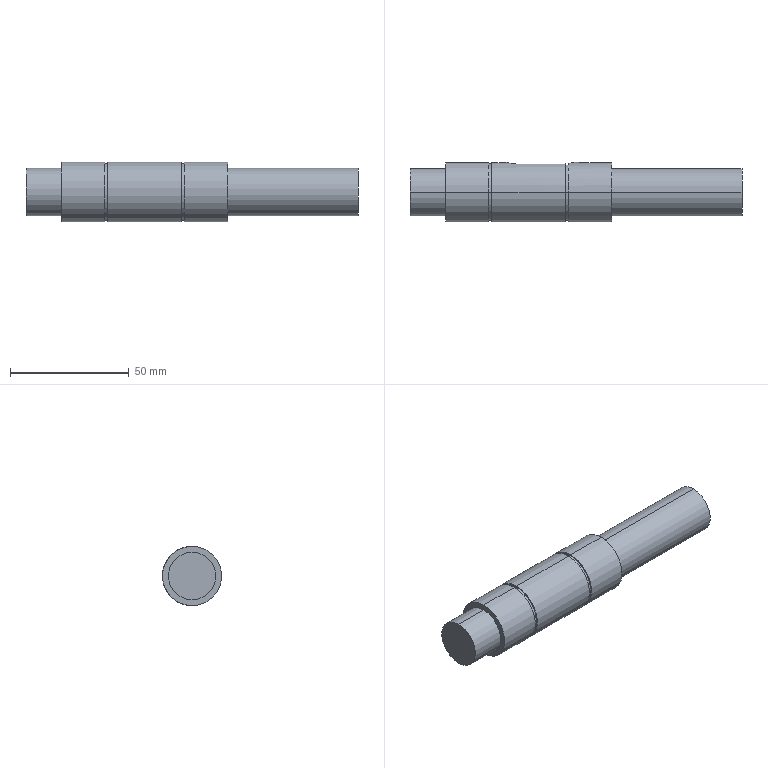Part | SolidWorks | features ICE 3, Extrusion 1, RevCut 1 | 1 solid | 28 faces | box 140 x 25 x 25 mm | volume 55450 mm3 | cylinder 17 | plane 11 | commonest cylinder face diameters 25 x6 23.9 x5 20 x4 8 x2
STEP:
#1=CARTESIAN_POINT('',(-50.,0.,10.));
#2=VERTEX_POINT('',#1);
#3=CARTESIAN_POINT('',(-50.,0.,-10.));
#4=VERTEX_POINT('',#3);
#5=CARTESIAN_POINT('',(-50.,0.,0.));
#6=DIRECTION('',(-1.,0.,0.));
#7=DIRECTION('',(0.,0.,1.));
#8=AXIS2_PLACEMENT_3D('',#5,#6,#7);
#9=CIRCLE('',#8,10.);
#10=EDGE_CURVE('',#2,#4,#9,.T.);
#11=ORIENTED_EDGE('',*,*,#10,.F.);
#12=CARTESIAN_POINT('',(-35.,0.,10.));
#13=VERTEX_POINT('',#12);
#14=CARTESIAN_POINT('',(-50.,0.,10.));
#15=DIRECTION('',(1.,0.,0.));
#16=VECTOR('',#15,1000.);
#17=LINE('',#14,#16);
#18=EDGE_CURVE('',#2,#13,#17,.T.);
#19=ORIENTED_EDGE('',*,*,#18,.T.);
#20=CARTESIAN_POINT('',(-35.,0.,-10.));
#21=VERTEX_POINT('',#20);
#22=CARTESIAN_POINT('',(-35.,0.,0.));
#23=DIRECTION('',(-1.,0.,0.));
#24=DIRECTION('',(0.,0.,1.));
#25=AXIS2_PLACEMENT_3D('',#22,#23,#24);
#26=CIRCLE('',#25,10.);
#27=EDGE_CURVE('',#13,#21,#26,.T.);
#28=ORIENTED_EDGE('',*,*,#27,.T.);
#29=CARTESIAN_POINT('',(-50.,0.,-10.));
#30=DIRECTION('',(1.,0.,0.));
#31=VECTOR('',#30,1000.);
#32=LINE('',#29,#31);
#33=EDGE_CURVE('',#4,#21,#32,.T.);
#34=ORIENTED_EDGE('',*,*,#33,.F.);
#35=EDGE_LOOP('',(#11,#19,#28,#34));
#36=FACE_OUTER_BOUND('',#35,.T.);
#37=CARTESIAN_POINT('',(-50.,0.,0.));
#38=DIRECTION('',(1.,0.,0.));
#39=DIRECTION('',(0.,0.,-1.));
#40=AXIS2_PLACEMENT_3D('',#37,#38,#39);
#41=CYLINDRICAL_SURFACE('',#40,10.);
#42=ADVANCED_FACE('',(#36),#41,.T.);
#43=CARTESIAN_POINT('',(-16.8,0.,12.5));
#44=VERTEX_POINT('',#43);
#45=CARTESIAN_POINT('',(-16.8,0.,-12.5));
#46=VERTEX_POINT('',#45);
#47=CARTESIAN_POINT('',(-16.8,0.,0.));
#48=DIRECTION('',(-1.,0.,0.));
#49=DIRECTION('',(0.,0.,1.));
#50=AXIS2_PLACEMENT_3D('',#47,#48,#49);
#51=CIRCLE('',#50,12.5);
#52=EDGE_CURVE('',#44,#46,#51,.T.);
#53=ORIENTED_EDGE('',*,*,#52,.T.);
#54=CARTESIAN_POINT('',(-35.,0.,-12.5));
#55=VERTEX_POINT('',#54);
#56=CARTESIAN_POINT('',(35.,0.,-12.5));
#57=DIRECTION('',(-1.,0.,0.));
#58=VECTOR('',#57,1000.);
#59=LINE('',#56,#58);
#60=EDGE_CURVE('',#46,#55,#59,.T.);
#61=ORIENTED_EDGE('',*,*,#60,.T.);
#62=CARTESIAN_POINT('',(-35.,0.,12.5));
#63=VERTEX_POINT('',#62);
#64=CARTESIAN_POINT('',(-35.,0.,0.));
#65=DIRECTION('',(1.,0.,0.));
#66=DIRECTION('',(0.,0.,-1.));
#67=AXIS2_PLACEMENT_3D('',#64,#65,#66);
#68=CIRCLE('',#67,12.5);
#69=EDGE_CURVE('',#55,#63,#68,.T.);
#70=ORIENTED_EDGE('',*,*,#69,.T.);
#71=CARTESIAN_POINT('',(35.,0.,12.5));
#72=DIRECTION('',(-1.,0.,0.));
#73=VECTOR('',#72,1000.);
#74=LINE('',#71,#73);
#75=EDGE_CURVE('',#44,#63,#74,.T.);
#76=ORIENTED_EDGE('',*,*,#75,.F.);
#77=EDGE_LOOP('',(#53,#61,#70,#76));
#78=FACE_OUTER_BOUND('',#77,.T.);
#79=CARTESIAN_POINT('',(35.,0.,0.));
#80=DIRECTION('',(-1.,0.,0.));
#81=DIRECTION('',(0.,0.,1.));
#82=AXIS2_PLACEMENT_3D('',#79,#80,#81);
#83=CYLINDRICAL_SURFACE('',#82,12.5);
#84=ADVANCED_FACE('',(#78),#83,.T.);
#85=CARTESIAN_POINT('',(-15.5,0.,11.95));
#86=VERTEX_POINT('',#85);
#87=CARTESIAN_POINT('',(-15.5,0.,-11.95));
#88=VERTEX_POINT('',#87);
#89=CARTESIAN_POINT('',(-15.5,0.,0.));
#90=DIRECTION('',(-1.,0.,0.));
#91=DIRECTION('',(0.,0.,1.));
#92=AXIS2_PLACEMENT_3D('',#89,#90,#91);
#93=CIRCLE('',#92,11.95);
#94=EDGE_CURVE('',#86,#88,#93,.T.);
#95=ORIENTED_EDGE('',*,*,#94,.T.);
#96=CARTESIAN_POINT('',(-16.8,0.,-11.95));
#97=VERTEX_POINT('',#96);
#98=CARTESIAN_POINT('',(0.,0.,-11.95));
#99=DIRECTION('',(-1.,0.,0.));
#100=VECTOR('',#99,1000.);
#101=LINE('',#98,#100);
#102=EDGE_CURVE('',#88,#97,#101,.T.);
#103=ORIENTED_EDGE('',*,*,#102,.T.);
#104=CARTESIAN_POINT('',(-16.8,0.,11.95));
#105=VERTEX_POINT('',#104);
#106=CARTESIAN_POINT('',(-16.8,0.,0.));
#107=DIRECTION('',(-1.,0.,0.));
#108=DIRECTION('',(0.,0.,1.));
#109=AXIS2_PLACEMENT_3D('',#106,#107,#108);
#110=CIRCLE('',#109,11.95);
#111=EDGE_CURVE('',#105,#97,#110,.T.);
#112=ORIENTED_EDGE('',*,*,#111,.F.);
#113=CARTESIAN_POINT('',(0.,0.,11.95));
#114=DIRECTION('',(-1.,0.,0.));
#115=VECTOR('',#114,1000.);
#116=LINE('',#113,#115);
#117=EDGE_CURVE('',#86,#105,#116,.T.);
#118=ORIENTED_EDGE('',*,*,#117,.F.);
#119=EDGE_LOOP('',(#95,#103,#112,#118));
#120=FACE_OUTER_BOUND('',#119,.T.);
#121=CARTESIAN_POINT('',(0.,0.,0.));
#122=DIRECTION('',(-1.,0.,0.));
#123=DIRECTION('',(0.,0.,1.));
#124=AXIS2_PLACEMENT_3D('',#121,#122,#123);
#125=CYLINDRICAL_SURFACE('',#124,11.95);
#126=ADVANCED_FACE('',(#120),#125,.T.);
#127=CARTESIAN_POINT('',(90.,0.,-10.));
#128=VERTEX_POINT('',#127);
#129=CARTESIAN_POINT('',(90.,0.,10.));
#130=VERTEX_POINT('',#129);
#131=CARTESIAN_POINT('',(90.,0.,0.));
#132=DIRECTION('',(1.,0.,0.));
#133=DIRECTION('',(0.,0.,-1.));
#134=AXIS2_PLACEMENT_3D('',#131,#132,#133);
#135=CIRCLE('',#134,10.);
#136=EDGE_CURVE('',#128,#130,#135,.T.);
#137=ORIENTED_EDGE('',*,*,#136,.F.);
#138=CARTESIAN_POINT('',(35.,0.,-10.));
#139=VERTEX_POINT('',#138);
#140=CARTESIAN_POINT('',(90.,0.,-10.));
#141=DIRECTION('',(-1.,0.,0.));
#142=VECTOR('',#141,1000.);
#143=LINE('',#140,#142);
#144=EDGE_CURVE('',#128,#139,#143,.T.);
#145=ORIENTED_EDGE('',*,*,#144,.T.);
#146=CARTESIAN_POINT('',(35.,0.,10.));
#147=VERTEX_POINT('',#146);
#148=CARTESIAN_POINT('',(35.,0.,0.));
#149=DIRECTION('',(1.,0.,0.));
#150=DIRECTION('',(0.,0.,-1.));
#151=AXIS2_PLACEMENT_3D('',#148,#149,#150);
#152=CIRCLE('',#151,10.);
#153=EDGE_CURVE('',#139,#147,#152,.T.);
#154=ORIENTED_EDGE('',*,*,#153,.T.);
#155=CARTESIAN_POINT('',(90.,0.,10.));
#156=DIRECTION('',(-1.,0.,0.));
#157=VECTOR('',#156,1000.);
#158=LINE('',#155,#157);
#159=EDGE_CURVE('',#130,#147,#158,.T.);
#160=ORIENTED_EDGE('',*,*,#159,.F.);
#161=EDGE_LOOP('',(#137,#145,#154,#160));
#162=FACE_OUTER_BOUND('',#161,.T.);
#163=CARTESIAN_POINT('',(90.,0.,0.));
#164=DIRECTION('',(-1.,0.,0.));
#165=DIRECTION('',(0.,0.,1.));
#166=AXIS2_PLACEMENT_3D('',#163,#164,#165);
#167=CYLINDRICAL_SURFACE('',#166,10.);
#168=ADVANCED_FACE('',(#162),#167,.T.);
#169=CARTESIAN_POINT('',(15.5,11.853,-3.969));
#170=VERTEX_POINT('',#169);
#171=CARTESIAN_POINT('',(15.5,0.,-12.5));
#172=VERTEX_POINT('',#171);
#173=CARTESIAN_POINT('',(15.5,0.,0.));
#174=DIRECTION('',(-1.,0.,0.));
#175=DIRECTION('',(0.,0.,1.));
#176=AXIS2_PLACEMENT_3D('',#173,#174,#175);
#177=CIRCLE('',#176,12.5);
#178=EDGE_CURVE('',#170,#172,#177,.T.);
#179=ORIENTED_EDGE('',*,*,#178,.T.);
#180=CARTESIAN_POINT('',(-15.5,0.,-12.5));
#181=VERTEX_POINT('',#180);
#182=CARTESIAN_POINT('',(35.,0.,-12.5));
#183=DIRECTION('',(-1.,0.,0.));
#184=VECTOR('',#183,1000.);
#185=LINE('',#182,#184);
#186=EDGE_CURVE('',#172,#181,#185,.T.);
#187=ORIENTED_EDGE('',*,*,#186,.T.);
#188=CARTESIAN_POINT('',(-15.5,0.,12.5));
#189=VERTEX_POINT('',#188);
#190=CARTESIAN_POINT('',(-15.5,0.,0.));
#191=DIRECTION('',(-1.,0.,0.));
#192=DIRECTION('',(0.,0.,1.));
#193=AXIS2_PLACEMENT_3D('',#190,#191,#192);
#194=CIRCLE('',#193,12.5);
#195=EDGE_CURVE('',#189,#181,#194,.T.);
#196=ORIENTED_EDGE('',*,*,#195,.F.);
#197=CARTESIAN_POINT('',(15.5,0.,12.5));
#198=VERTEX_POINT('',#197);
#199=CARTESIAN_POINT('',(35.,0.,12.5));
#200=DIRECTION('',(-1.,0.,0.));
#201=VECTOR('',#200,1000.);
#202=LINE('',#199,#201);
#203=EDGE_CURVE('',#198,#189,#202,.T.);
#204=ORIENTED_EDGE('',*,*,#203,.F.);
#205=CARTESIAN_POINT('',(15.5,11.853,3.969));
#206=VERTEX_POINT('',#205);
#207=CARTESIAN_POINT('',(15.5,0.,0.));
#208=DIRECTION('',(-1.,0.,0.));
#209=DIRECTION('',(0.,0.,1.));
#210=AXIS2_PLACEMENT_3D('',#207,#208,#209);
#211=CIRCLE('',#210,12.5);
#212=EDGE_CURVE('',#198,#206,#211,.T.);
#213=ORIENTED_EDGE('',*,*,#212,.T.);
#214=CARTESIAN_POINT('',(15.,11.843,4.));
#215=VERTEX_POINT('',#214);
#216=CARTESIAN_POINT('',(15.,11.843,4.));
#217=CARTESIAN_POINT('',(15.167,11.843,4.));
#218=CARTESIAN_POINT('',(15.334,11.846,3.99));
#219=CARTESIAN_POINT('',(15.5,11.853,3.969));
#220=B_SPLINE_CURVE_WITH_KNOTS('',3,(#216,#217,#218,#219),.UNSPECIFIED.,.F.,.F.,(4,4),(0.,0.0005011),.UNSPECIFIED.);
#221=EDGE_CURVE('',#215,#206,#220,.T.);
#222=ORIENTED_EDGE('',*,*,#221,.F.);
#223=CARTESIAN_POINT('',(-5.,11.843,4.));
#224=VERTEX_POINT('',#223);
#225=CARTESIAN_POINT('',(35.,11.843,4.));
#226=DIRECTION('',(1.,0.,0.));
#227=VECTOR('',#226,1000.);
#228=LINE('',#225,#227);
#229=EDGE_CURVE('',#224,#215,#228,.T.);
#230=ORIENTED_EDGE('',*,*,#229,.F.);
#231=CARTESIAN_POINT('',(-5.,11.843,-4.));
#232=VERTEX_POINT('',#231);
#233=CARTESIAN_POINT('',(-5.,11.843,-4.));
#234=CARTESIAN_POINT('',(-5.266,11.843,-4.));
#235=CARTESIAN_POINT('',(-5.527,11.852,-3.974));
#236=CARTESIAN_POINT('',(-6.041,11.886,-3.871));
#237=CARTESIAN_POINT('',(-6.296,11.911,-3.793));
#238=CARTESIAN_POINT('',(-6.779,11.973,-3.592));
#239=CARTESIAN_POINT('',(-7.008,12.01,-3.469));
#240=CARTESIAN_POINT('',(-7.441,12.09,-3.179));
#241=CARTESIAN_POINT('',(-7.645,12.133,-3.012));
#242=CARTESIAN_POINT('',(-8.011,12.218,-2.646));
#243=CARTESIAN_POINT('',(-8.176,12.26,-2.445));
#244=CARTESIAN_POINT('',(-8.469,12.34,-2.009));
#245=CARTESIAN_POINT('',(-8.592,12.375,-1.779));
#246=CARTESIAN_POINT('',(-8.792,12.435,-1.299));
#247=CARTESIAN_POINT('',(-8.87,12.459,-1.045));
#248=CARTESIAN_POINT('',(-8.974,12.492,-0.5276));
#249=CARTESIAN_POINT('',(-9.,12.5,-0.2669));
#250=CARTESIAN_POINT('',(-9.,12.5,0.2587));
#251=CARTESIAN_POINT('',(-8.974,12.492,0.5256));
#252=CARTESIAN_POINT('',(-8.871,12.459,1.04));
#253=CARTESIAN_POINT('',(-8.795,12.436,1.29));
#254=CARTESIAN_POINT('',(-8.593,12.375,1.777));
#255=CARTESIAN_POINT('',(-8.469,12.34,2.008));
#256=CARTESIAN_POINT('',(-8.18,12.262,2.44));
#257=CARTESIAN_POINT('',(-8.013,12.219,2.643));
#258=CARTESIAN_POINT('',(-7.645,12.133,3.012));
#259=CARTESIAN_POINT('',(-7.445,12.091,3.176));
#260=CARTESIAN_POINT('',(-7.013,12.011,3.466));
#261=CARTESIAN_POINT('',(-6.78,11.973,3.592));
#262=CARTESIAN_POINT('',(-6.298,11.911,3.792));
#263=CARTESIAN_POINT('',(-6.049,11.886,3.869));
#264=CARTESIAN_POINT('',(-5.532,11.852,3.973));
#265=CARTESIAN_POINT('',(-5.266,11.843,4.));
#266=CARTESIAN_POINT('',(-5.,11.843,4.));
#267=B_SPLINE_CURVE_WITH_KNOTS('',3,(#233,#234,#235,#236,#237,#238,#239,#240,#241,#242,#243,#244,#245,#246,#247,#248,#249,#250,#251,#252,#253,#254,#255,#256,#257,#258,#259,#260,#261,#262,#263,#264,#265,#266),.UNSPECIFIED.,.F.,.F.,(4,2,2,2,2,2,2,2,2,2,2,2,2,2,2,2,4),(0.,0.0007865,0.001573,0.00236,0.003146,0.003933,0.004719,0.005506,0.006292,0.007079,0.007865,0.008652,0.009438,0.01022,0.01101,0.0118,0.01258),.UNSPECIFIED.);
#268=EDGE_CURVE('',#232,#224,#267,.T.);
#269=ORIENTED_EDGE('',*,*,#268,.F.);
#270=CARTESIAN_POINT('',(15.,11.843,-4.));
#271=VERTEX_POINT('',#270);
#272=CARTESIAN_POINT('',(35.,11.843,-4.));
#273=DIRECTION('',(-1.,0.,0.));
#274=VECTOR('',#273,1000.);
#275=LINE('',#272,#274);
#276=EDGE_CURVE('',#271,#232,#275,.T.);
#277=ORIENTED_EDGE('',*,*,#276,.F.);
#278=CARTESIAN_POINT('',(15.5,11.853,-3.969));
#279=CARTESIAN_POINT('',(15.334,11.846,-3.99));
#280=CARTESIAN_POINT('',(15.167,11.843,-4.));
#281=CARTESIAN_POINT('',(15.,11.843,-4.));
#282=B_SPLINE_CURVE_WITH_KNOTS('',3,(#278,#279,#280,#281),.UNSPECIFIED.,.F.,.F.,(4,4),(0.,0.0005011),.UNSPECIFIED.);
#283=EDGE_CURVE('',#170,#271,#282,.T.);
#284=ORIENTED_EDGE('',*,*,#283,.F.);
#285=EDGE_LOOP('',(#179,#187,#196,#204,#213,#222,#230,#269,#277,#284));
#286=FACE_OUTER_BOUND('',#285,.T.);
#287=CARTESIAN_POINT('',(35.,0.,0.));
#288=DIRECTION('',(-1.,0.,0.));
#289=DIRECTION('',(0.,0.,1.));
#290=AXIS2_PLACEMENT_3D('',#287,#288,#289);
#291=CYLINDRICAL_SURFACE('',#290,12.5);
#292=ADVANCED_FACE('',(#286),#291,.T.);
#293=CARTESIAN_POINT('',(16.8,11.404,-3.572));
#294=VERTEX_POINT('',#293);
#295=CARTESIAN_POINT('',(16.8,0.,-11.95));
#296=VERTEX_POINT('',#295);
#297=CARTESIAN_POINT('',(16.8,0.,0.));
#298=DIRECTION('',(-1.,0.,0.));
#299=DIRECTION('',(0.,0.,1.));
#300=AXIS2_PLACEMENT_3D('',#297,#298,#299);
#301=CIRCLE('',#300,11.95);
#302=EDGE_CURVE('',#294,#296,#301,.T.);
#303=ORIENTED_EDGE('',*,*,#302,.T.);
#304=CARTESIAN_POINT('',(15.5,0.,-11.95));
#305=VERTEX_POINT('',#304);
#306=CARTESIAN_POINT('',(0.,0.,-11.95));
#307=DIRECTION('',(-1.,0.,0.));
#308=VECTOR('',#307,1000.);
#309=LINE('',#306,#308);
#310=EDGE_CURVE('',#296,#305,#309,.T.);
#311=ORIENTED_EDGE('',*,*,#310,.T.);
#312=CARTESIAN_POINT('',(15.5,11.272,-3.969));
#313=VERTEX_POINT('',#312);
#314=CARTESIAN_POINT('',(15.5,0.,0.));
#315=DIRECTION('',(-1.,0.,0.));
#316=DIRECTION('',(0.,0.,1.));
#317=AXIS2_PLACEMENT_3D('',#314,#315,#316);
#318=CIRCLE('',#317,11.95);
#319=EDGE_CURVE('',#313,#305,#318,.T.);
#320=ORIENTED_EDGE('',*,*,#319,.F.);
#321=CARTESIAN_POINT('',(15.5,11.272,-3.969));
#322=CARTESIAN_POINT('',(15.958,11.292,-3.911));
#323=CARTESIAN_POINT('',(16.391,11.339,-3.778));
#324=CARTESIAN_POINT('',(16.8,11.404,-3.572));
#325=B_SPLINE_CURVE_WITH_KNOTS('',3,(#321,#322,#323,#324),.UNSPECIFIED.,.F.,.F.,(4,4),(0.,0.001366),.UNSPECIFIED.);
#326=EDGE_CURVE('',#313,#294,#325,.T.);
#327=ORIENTED_EDGE('',*,*,#326,.T.);
#328=EDGE_LOOP('',(#303,#311,#320,#327));
#329=FACE_OUTER_BOUND('',#328,.T.);
#330=CARTESIAN_POINT('',(0.,0.,0.));
#331=DIRECTION('',(-1.,0.,0.));
#332=DIRECTION('',(0.,0.,1.));
#333=AXIS2_PLACEMENT_3D('',#330,#331,#332);
#334=CYLINDRICAL_SURFACE('',#333,11.95);
#335=ADVANCED_FACE('',(#329),#334,.T.);
#336=ORIENTED_EDGE('',*,*,#310,.F.);
#337=CARTESIAN_POINT('',(16.8,0.,11.95));
#338=VERTEX_POINT('',#337);
#339=CARTESIAN_POINT('',(16.8,0.,0.));
#340=DIRECTION('',(-1.,0.,0.));
#341=DIRECTION('',(0.,0.,1.));
#342=AXIS2_PLACEMENT_3D('',#339,#340,#341);
#343=CIRCLE('',#342,11.95);
#344=EDGE_CURVE('',#296,#338,#343,.T.);
#345=ORIENTED_EDGE('',*,*,#344,.T.);
#346=CARTESIAN_POINT('',(15.5,0.,11.95));
#347=VERTEX_POINT('',#346);
#348=CARTESIAN_POINT('',(0.,0.,11.95));
#349=DIRECTION('',(-1.,0.,0.));
#350=VECTOR('',#349,1000.);
#351=LINE('',#348,#350);
#352=EDGE_CURVE('',#338,#347,#351,.T.);
#353=ORIENTED_EDGE('',*,*,#352,.T.);
#354=CARTESIAN_POINT('',(15.5,0.,0.));
#355=DIRECTION('',(-1.,0.,0.));
#356=DIRECTION('',(0.,0.,1.));
#357=AXIS2_PLACEMENT_3D('',#354,#355,#356);
#358=CIRCLE('',#357,11.95);
#359=EDGE_CURVE('',#305,#347,#358,.T.);
#360=ORIENTED_EDGE('',*,*,#359,.F.);
#361=EDGE_LOOP('',(#336,#345,#353,#360));
#362=FACE_OUTER_BOUND('',#361,.T.);
#363=CARTESIAN_POINT('',(0.,0.,0.));
#364=DIRECTION('',(-1.,0.,0.));
#365=DIRECTION('',(0.,0.,1.));
#366=AXIS2_PLACEMENT_3D('',#363,#364,#365);
#367=CYLINDRICAL_SURFACE('',#366,11.95);
#368=ADVANCED_FACE('',(#362),#367,.T.);
#369=CARTESIAN_POINT('',(35.,0.,-12.5));
#370=VERTEX_POINT('',#369);
#371=CARTESIAN_POINT('',(35.,0.,12.5));
#372=VERTEX_POINT('',#371);
#373=CARTESIAN_POINT('',(35.,0.,0.));
#374=DIRECTION('',(1.,0.,0.));
#375=DIRECTION('',(0.,0.,-1.));
#376=AXIS2_PLACEMENT_3D('',#373,#374,#375);
#377=CIRCLE('',#376,12.5);
#378=EDGE_CURVE('',#370,#372,#377,.T.);
#379=ORIENTED_EDGE('',*,*,#378,.F.);
#380=CARTESIAN_POINT('',(16.8,0.,-12.5));
#381=VERTEX_POINT('',#380);
#382=CARTESIAN_POINT('',(35.,0.,-12.5));
#383=DIRECTION('',(-1.,0.,0.));
#384=VECTOR('',#383,1000.);
#385=LINE('',#382,#384);
#386=EDGE_CURVE('',#370,#381,#385,.T.);
#387=ORIENTED_EDGE('',*,*,#386,.T.);
#388=CARTESIAN_POINT('',(16.8,11.979,-3.572));
#389=VERTEX_POINT('',#388);
#390=CARTESIAN_POINT('',(16.8,0.,0.));
#391=DIRECTION('',(-1.,0.,0.));
#392=DIRECTION('',(0.,0.,1.));
#393=AXIS2_PLACEMENT_3D('',#390,#391,#392);
#394=CIRCLE('',#393,12.5);
#395=EDGE_CURVE('',#389,#381,#394,.T.);
#396=ORIENTED_EDGE('',*,*,#395,.F.);
#397=CARTESIAN_POINT('',(16.8,11.979,3.572));
#398=VERTEX_POINT('',#397);
#399=CARTESIAN_POINT('',(16.8,11.979,3.572));
#400=CARTESIAN_POINT('',(17.131,12.029,3.405));
#401=CARTESIAN_POINT('',(17.431,12.087,3.198));
#402=CARTESIAN_POINT('',(17.836,12.177,2.827));
#403=CARTESIAN_POINT('',(17.964,12.207,2.692));
#404=CARTESIAN_POINT('',(18.197,12.266,2.411));
#405=CARTESIAN_POINT('',(18.304,12.295,2.262));
#406=CARTESIAN_POINT('',(18.592,12.374,1.797));
#407=CARTESIAN_POINT('',(18.745,12.42,1.453));
#408=CARTESIAN_POINT('',(18.896,12.467,0.9231));
#409=CARTESIAN_POINT('',(18.935,12.479,0.743));
#410=CARTESIAN_POINT('',(18.987,12.496,0.3759));
#411=CARTESIAN_POINT('',(19.,12.5,0.1881));
#412=CARTESIAN_POINT('',(19.,12.5,-0.1823));
#413=CARTESIAN_POINT('',(18.987,12.496,-0.3664));
#414=CARTESIAN_POINT('',(18.937,12.48,-0.7322));
#415=CARTESIAN_POINT('',(18.898,12.468,-0.9152));
#416=CARTESIAN_POINT('',(18.746,12.421,-1.451));
#417=CARTESIAN_POINT('',(18.598,12.376,-1.786));
#418=CARTESIAN_POINT('',(18.21,12.269,-2.416));
#419=CARTESIAN_POINT('',(17.976,12.208,-2.698));
#420=CARTESIAN_POINT('',(17.572,12.118,-3.069));
#421=CARTESIAN_POINT('',(17.427,12.088,-3.185));
#422=CARTESIAN_POINT('',(17.124,12.031,-3.394));
#423=CARTESIAN_POINT('',(16.966,12.004,-3.489));
#424=CARTESIAN_POINT('',(16.8,11.979,-3.572));
#425=B_SPLINE_CURVE_WITH_KNOTS('',3,(#399,#400,#401,#402,#403,#404,#405,#406,#407,#408,#409,#410,#411,#412,#413,#414,#415,#416,#417,#418,#419,#420,#421,#422,#423,#424),.UNSPECIFIED.,.F.,.F.,(4,2,2,2,2,2,2,2,2,2,2,2,4),(0.,0.001107,0.00166,0.002214,0.00332,0.003874,0.004427,0.004981,0.005534,0.006641,0.007748,0.008301,0.008855),.UNSPECIFIED.);
#426=EDGE_CURVE('',#398,#389,#425,.T.);
#427=ORIENTED_EDGE('',*,*,#426,.F.);
#428=CARTESIAN_POINT('',(16.8,0.,12.5));
#429=VERTEX_POINT('',#428);
#430=CARTESIAN_POINT('',(16.8,0.,0.));
#431=DIRECTION('',(-1.,0.,0.));
#432=DIRECTION('',(0.,0.,1.));
#433=AXIS2_PLACEMENT_3D('',#430,#431,#432);
#434=CIRCLE('',#433,12.5);
#435=EDGE_CURVE('',#429,#398,#434,.T.);
#436=ORIENTED_EDGE('',*,*,#435,.F.);
#437=CARTESIAN_POINT('',(35.,0.,12.5));
#438=DIRECTION('',(-1.,0.,0.));
#439=VECTOR('',#438,1000.);
#440=LINE('',#437,#439);
#441=EDGE_CURVE('',#372,#429,#440,.T.);
#442=ORIENTED_EDGE('',*,*,#441,.F.);
#443=EDGE_LOOP('',(#379,#387,#396,#427,#436,#442));
#444=FACE_OUTER_BOUND('',#443,.T.);
#445=CARTESIAN_POINT('',(35.,0.,0.));
#446=DIRECTION('',(-1.,0.,0.));
#447=DIRECTION('',(0.,0.,1.));
#448=AXIS2_PLACEMENT_3D('',#445,#446,#447);
#449=CYLINDRICAL_SURFACE('',#448,12.5);
#450=ADVANCED_FACE('',(#444),#449,.T.);
#451=ORIENTED_EDGE('',*,*,#386,.F.);
#452=CARTESIAN_POINT('',(35.,0.,0.));
#453=DIRECTION('',(1.,0.,0.));
#454=DIRECTION('',(0.,0.,-1.));
#455=AXIS2_PLACEMENT_3D('',#452,#453,#454);
#456=CIRCLE('',#455,12.5);
#457=EDGE_CURVE('',#372,#370,#456,.T.);
#458=ORIENTED_EDGE('',*,*,#457,.F.);
#459=ORIENTED_EDGE('',*,*,#441,.T.);
#460=CARTESIAN_POINT('',(16.8,0.,0.));
#461=DIRECTION('',(-1.,0.,0.));
#462=DIRECTION('',(0.,0.,1.));
#463=AXIS2_PLACEMENT_3D('',#460,#461,#462);
#464=CIRCLE('',#463,12.5);
#465=EDGE_CURVE('',#381,#429,#464,.T.);
#466=ORIENTED_EDGE('',*,*,#465,.F.);
#467=EDGE_LOOP('',(#451,#458,#459,#466));
#468=FACE_OUTER_BOUND('',#467,.T.);
#469=CARTESIAN_POINT('',(35.,0.,0.));
#470=DIRECTION('',(-1.,0.,0.));
#471=DIRECTION('',(0.,0.,1.));
#472=AXIS2_PLACEMENT_3D('',#469,#470,#471);
#473=CYLINDRICAL_SURFACE('',#472,12.5);
#474=ADVANCED_FACE('',(#468),#473,.T.);
#475=ORIENTED_EDGE('',*,*,#319,.T.);
#476=ORIENTED_EDGE('',*,*,#359,.T.);
#477=CARTESIAN_POINT('',(15.5,11.272,3.969));
#478=VERTEX_POINT('',#477);
#479=CARTESIAN_POINT('',(15.5,0.,0.));
#480=DIRECTION('',(-1.,0.,0.));
#481=DIRECTION('',(0.,0.,1.));
#482=AXIS2_PLACEMENT_3D('',#479,#480,#481);
#483=CIRCLE('',#482,11.95);
#484=EDGE_CURVE('',#347,#478,#483,.T.);
#485=ORIENTED_EDGE('',*,*,#484,.T.);
#486=CARTESIAN_POINT('',(15.5,12.5,3.969));
#487=DIRECTION('',(0.,1.,0.));
#488=VECTOR('',#487,1000.);
#489=LINE('',#486,#488);
#490=EDGE_CURVE('',#478,#206,#489,.T.);
#491=ORIENTED_EDGE('',*,*,#490,.T.);
#492=ORIENTED_EDGE('',*,*,#212,.F.);
#493=CARTESIAN_POINT('',(15.5,0.,0.));
#494=DIRECTION('',(-1.,0.,0.));
#495=DIRECTION('',(0.,0.,1.));
#496=AXIS2_PLACEMENT_3D('',#493,#494,#495);
#497=CIRCLE('',#496,12.5);
#498=EDGE_CURVE('',#172,#198,#497,.T.);
#499=ORIENTED_EDGE('',*,*,#498,.F.);
#500=ORIENTED_EDGE('',*,*,#178,.F.);
#501=CARTESIAN_POINT('',(15.5,12.5,-3.969));
#502=DIRECTION('',(0.,-1.,0.));
#503=VECTOR('',#502,1000.);
#504=LINE('',#501,#503);
#505=EDGE_CURVE('',#170,#313,#504,.T.);
#506=ORIENTED_EDGE('',*,*,#505,.T.);
#507=EDGE_LOOP('',(#475,#476,#485,#491,#492,#499,#500,#506));
#508=FACE_OUTER_BOUND('',#507,.T.);
#509=CARTESIAN_POINT('',(15.5,0.,-12.5));
#510=DIRECTION('',(1.,0.,0.));
#511=DIRECTION('',(0.,0.,-1.));
#512=AXIS2_PLACEMENT_3D('',#509,#510,#511);
#513=PLANE('',#512);
#514=ADVANCED_FACE('',(#508),#513,.T.);
#515=ORIENTED_EDGE('',*,*,#352,.F.);
#516=CARTESIAN_POINT('',(16.8,11.404,3.572));
#517=VERTEX_POINT('',#516);
#518=CARTESIAN_POINT('',(16.8,0.,0.));
#519=DIRECTION('',(-1.,0.,0.));
#520=DIRECTION('',(0.,0.,1.));
#521=AXIS2_PLACEMENT_3D('',#518,#519,#520);
#522=CIRCLE('',#521,11.95);
#523=EDGE_CURVE('',#338,#517,#522,.T.);
#524=ORIENTED_EDGE('',*,*,#523,.T.);
#525=CARTESIAN_POINT('',(16.8,11.404,3.572));
#526=CARTESIAN_POINT('',(16.391,11.339,3.778));
#527=CARTESIAN_POINT('',(15.958,11.292,3.911));
#528=CARTESIAN_POINT('',(15.5,11.272,3.969));
#529=B_SPLINE_CURVE_WITH_KNOTS('',3,(#525,#526,#527,#528),.UNSPECIFIED.,.F.,.F.,(4,4),(0.,0.001366),.UNSPECIFIED.);
#530=EDGE_CURVE('',#517,#478,#529,.T.);
#531=ORIENTED_EDGE('',*,*,#530,.T.);
#532=ORIENTED_EDGE('',*,*,#484,.F.);
#533=EDGE_LOOP('',(#515,#524,#531,#532));
#534=FACE_OUTER_BOUND('',#533,.T.);
#535=CARTESIAN_POINT('',(0.,0.,0.));
#536=DIRECTION('',(-1.,0.,0.));
#537=DIRECTION('',(0.,0.,1.));
#538=AXIS2_PLACEMENT_3D('',#535,#536,#537);
#539=CYLINDRICAL_SURFACE('',#538,11.95);
#540=ADVANCED_FACE('',(#534),#539,.T.);
#541=ORIENTED_EDGE('',*,*,#302,.F.);
#542=CARTESIAN_POINT('',(16.8,12.5,-3.572));
#543=DIRECTION('',(0.,1.,0.));
#544=VECTOR('',#543,1000.);
#545=LINE('',#542,#544);
#546=EDGE_CURVE('',#294,#389,#545,.T.);
#547=ORIENTED_EDGE('',*,*,#546,.T.);
#548=ORIENTED_EDGE('',*,*,#395,.T.);
#549=ORIENTED_EDGE('',*,*,#465,.T.);
#550=ORIENTED_EDGE('',*,*,#435,.T.);
#551=CARTESIAN_POINT('',(16.8,12.5,3.572));
#552=DIRECTION('',(0.,-1.,0.));
#553=VECTOR('',#552,1000.);
#554=LINE('',#551,#553);
#555=EDGE_CURVE('',#398,#517,#554,.T.);
#556=ORIENTED_EDGE('',*,*,#555,.T.);
#557=ORIENTED_EDGE('',*,*,#523,.F.);
#558=ORIENTED_EDGE('',*,*,#344,.F.);
#559=EDGE_LOOP('',(#541,#547,#548,#549,#550,#556,#557,#558));
#560=FACE_OUTER_BOUND('',#559,.T.);
#561=CARTESIAN_POINT('',(16.8,0.,-12.5));
#562=DIRECTION('',(-1.,0.,0.));
#563=DIRECTION('',(0.,0.,1.));
#564=AXIS2_PLACEMENT_3D('',#561,#562,#563);
#565=PLANE('',#564);
#566=ADVANCED_FACE('',(#560),#565,.T.);
#567=ORIENTED_EDGE('',*,*,#186,.F.);
#568=ORIENTED_EDGE('',*,*,#498,.T.);
#569=ORIENTED_EDGE('',*,*,#203,.T.);
#570=CARTESIAN_POINT('',(-15.5,0.,0.));
#571=DIRECTION('',(-1.,0.,0.));
#572=DIRECTION('',(0.,0.,1.));
#573=AXIS2_PLACEMENT_3D('',#570,#571,#572);
#574=CIRCLE('',#573,12.5);
#575=EDGE_CURVE('',#181,#189,#574,.T.);
#576=ORIENTED_EDGE('',*,*,#575,.F.);
#577=EDGE_LOOP('',(#567,#568,#569,#576));
#578=FACE_OUTER_BOUND('',#577,.T.);
#579=CARTESIAN_POINT('',(35.,0.,0.));
#580=DIRECTION('',(-1.,0.,0.));
#581=DIRECTION('',(0.,0.,1.));
#582=AXIS2_PLACEMENT_3D('',#579,#580,#581);
#583=CYLINDRICAL_SURFACE('',#582,12.5);
#584=ADVANCED_FACE('',(#578),#583,.T.);
#585=CARTESIAN_POINT('',(35.,0.,0.));
#586=DIRECTION('',(1.,0.,0.));
#587=DIRECTION('',(0.,0.,-1.));
#588=AXIS2_PLACEMENT_3D('',#585,#586,#587);
#589=CIRCLE('',#588,10.);
#590=EDGE_CURVE('',#147,#139,#589,.T.);
#591=ORIENTED_EDGE('',*,*,#590,.F.);
#592=ORIENTED_EDGE('',*,*,#153,.F.);
#593=EDGE_LOOP('',(#591,#592));
#594=FACE_BOUND('',#593,.T.);
#595=ORIENTED_EDGE('',*,*,#457,.T.);
#596=ORIENTED_EDGE('',*,*,#378,.T.);
#597=EDGE_LOOP('',(#595,#596));
#598=FACE_OUTER_BOUND('',#597,.T.);
#599=CARTESIAN_POINT('',(35.,0.,0.));
#600=DIRECTION('',(1.,0.,0.));
#601=DIRECTION('',(0.,0.,-1.));
#602=AXIS2_PLACEMENT_3D('',#599,#600,#601);
#603=PLANE('',#602);
#604=ADVANCED_FACE('',(#594,#598),#603,.T.);
#605=ORIENTED_EDGE('',*,*,#144,.F.);
#606=CARTESIAN_POINT('',(90.,0.,0.));
#607=DIRECTION('',(1.,0.,0.));
#608=DIRECTION('',(0.,0.,-1.));
#609=AXIS2_PLACEMENT_3D('',#606,#607,#608);
#610=CIRCLE('',#609,10.);
#611=EDGE_CURVE('',#130,#128,#610,.T.);
#612=ORIENTED_EDGE('',*,*,#611,.F.);
#613=ORIENTED_EDGE('',*,*,#159,.T.);
#614=ORIENTED_EDGE('',*,*,#590,.T.);
#615=EDGE_LOOP('',(#605,#612,#613,#614));
#616=FACE_OUTER_BOUND('',#615,.T.);
#617=CARTESIAN_POINT('',(90.,0.,0.));
#618=DIRECTION('',(-1.,0.,0.));
#619=DIRECTION('',(0.,0.,1.));
#620=AXIS2_PLACEMENT_3D('',#617,#618,#619);
#621=CYLINDRICAL_SURFACE('',#620,10.);
#622=ADVANCED_FACE('',(#616),#621,.T.);
#623=ORIENTED_EDGE('',*,*,#611,.T.);
#624=ORIENTED_EDGE('',*,*,#136,.T.);
#625=EDGE_LOOP('',(#623,#624));
#626=FACE_OUTER_BOUND('',#625,.T.);
#627=CARTESIAN_POINT('',(90.,0.,0.));
#628=DIRECTION('',(1.,0.,0.));
#629=DIRECTION('',(0.,0.,-1.));
#630=AXIS2_PLACEMENT_3D('',#627,#628,#629);
#631=PLANE('',#630);
#632=ADVANCED_FACE('',(#626),#631,.T.);
#633=ORIENTED_EDGE('',*,*,#111,.T.);
#634=CARTESIAN_POINT('',(-16.8,0.,0.));
#635=DIRECTION('',(-1.,0.,0.));
#636=DIRECTION('',(0.,0.,1.));
#637=AXIS2_PLACEMENT_3D('',#634,#635,#636);
#638=CIRCLE('',#637,11.95);
#639=EDGE_CURVE('',#97,#105,#638,.T.);
#640=ORIENTED_EDGE('',*,*,#639,.T.);
#641=EDGE_LOOP('',(#633,#640));
#642=FACE_BOUND('',#641,.T.);
#643=ORIENTED_EDGE('',*,*,#52,.F.);
#644=CARTESIAN_POINT('',(-16.8,0.,0.));
#645=DIRECTION('',(-1.,0.,0.));
#646=DIRECTION('',(0.,0.,1.));
#647=AXIS2_PLACEMENT_3D('',#644,#645,#646);
#648=CIRCLE('',#647,12.5);
#649=EDGE_CURVE('',#46,#44,#648,.T.);
#650=ORIENTED_EDGE('',*,*,#649,.F.);
#651=EDGE_LOOP('',(#643,#650));
#652=FACE_OUTER_BOUND('',#651,.T.);
#653=CARTESIAN_POINT('',(-16.8,0.,-12.5));
#654=DIRECTION('',(1.,0.,0.));
#655=DIRECTION('',(0.,0.,-1.));
#656=AXIS2_PLACEMENT_3D('',#653,#654,#655);
#657=PLANE('',#656);
#658=ADVANCED_FACE('',(#642,#652),#657,.T.);
#659=ORIENTED_EDGE('',*,*,#102,.F.);
#660=CARTESIAN_POINT('',(-15.5,0.,0.));
#661=DIRECTION('',(-1.,0.,0.));
#662=DIRECTION('',(0.,0.,1.));
#663=AXIS2_PLACEMENT_3D('',#660,#661,#662);
#664=CIRCLE('',#663,11.95);
#665=EDGE_CURVE('',#88,#86,#664,.T.);
#666=ORIENTED_EDGE('',*,*,#665,.T.);
#667=ORIENTED_EDGE('',*,*,#117,.T.);
#668=ORIENTED_EDGE('',*,*,#639,.F.);
#669=EDGE_LOOP('',(#659,#666,#667,#668));
#670=FACE_OUTER_BOUND('',#669,.T.);
#671=CARTESIAN_POINT('',(0.,0.,0.));
#672=DIRECTION('',(-1.,0.,0.));
#673=DIRECTION('',(0.,0.,1.));
#674=AXIS2_PLACEMENT_3D('',#671,#672,#673);
#675=CYLINDRICAL_SURFACE('',#674,11.95);
#676=ADVANCED_FACE('',(#670),#675,.T.);
#677=ORIENTED_EDGE('',*,*,#195,.T.);
#678=ORIENTED_EDGE('',*,*,#575,.T.);
#679=EDGE_LOOP('',(#677,#678));
#680=FACE_OUTER_BOUND('',#679,.T.);
#681=ORIENTED_EDGE('',*,*,#94,.F.);
#682=ORIENTED_EDGE('',*,*,#665,.F.);
#683=EDGE_LOOP('',(#681,#682));
#684=FACE_BOUND('',#683,.T.);
#685=CARTESIAN_POINT('',(-15.5,0.,-12.5));
#686=DIRECTION('',(-1.,0.,0.));
#687=DIRECTION('',(0.,0.,1.));
#688=AXIS2_PLACEMENT_3D('',#685,#686,#687);
#689=PLANE('',#688);
#690=ADVANCED_FACE('',(#680,#684),#689,.T.);
#691=CARTESIAN_POINT('',(-35.,0.,0.));
#692=DIRECTION('',(-1.,0.,0.));
#693=DIRECTION('',(0.,0.,1.));
#694=AXIS2_PLACEMENT_3D('',#691,#692,#693);
#695=CIRCLE('',#694,10.);
#696=EDGE_CURVE('',#21,#13,#695,.T.);
#697=ORIENTED_EDGE('',*,*,#696,.F.);
#698=ORIENTED_EDGE('',*,*,#27,.F.);
#699=EDGE_LOOP('',(#697,#698));
#700=FACE_BOUND('',#699,.T.);
#701=CARTESIAN_POINT('',(-35.,0.,0.));
#702=DIRECTION('',(1.,0.,0.));
#703=DIRECTION('',(0.,0.,-1.));
#704=AXIS2_PLACEMENT_3D('',#701,#702,#703);
#705=CIRCLE('',#704,12.5);
#706=EDGE_CURVE('',#63,#55,#705,.T.);
#707=ORIENTED_EDGE('',*,*,#706,.F.);
#708=ORIENTED_EDGE('',*,*,#69,.F.);
#709=EDGE_LOOP('',(#707,#708));
#710=FACE_OUTER_BOUND('',#709,.T.);
#711=CARTESIAN_POINT('',(-35.,0.,0.));
#712=DIRECTION('',(1.,0.,0.));
#713=DIRECTION('',(0.,0.,-1.));
#714=AXIS2_PLACEMENT_3D('',#711,#712,#713);
#715=PLANE('',#714);
#716=ADVANCED_FACE('',(#700,#710),#715,.F.);
#717=ORIENTED_EDGE('',*,*,#60,.F.);
#718=ORIENTED_EDGE('',*,*,#649,.T.);
#719=ORIENTED_EDGE('',*,*,#75,.T.);
#720=ORIENTED_EDGE('',*,*,#706,.T.);
#721=EDGE_LOOP('',(#717,#718,#719,#720));
#722=FACE_OUTER_BOUND('',#721,.T.);
#723=CARTESIAN_POINT('',(35.,0.,0.));
#724=DIRECTION('',(-1.,0.,0.));
#725=DIRECTION('',(0.,0.,1.));
#726=AXIS2_PLACEMENT_3D('',#723,#724,#725);
#727=CYLINDRICAL_SURFACE('',#726,12.5);
#728=ADVANCED_FACE('',(#722),#727,.T.);
#729=CARTESIAN_POINT('',(-5.,8.5,-4.));
#730=VERTEX_POINT('',#729);
#731=CARTESIAN_POINT('',(-5.,12.5,-4.));
#732=DIRECTION('',(0.,-1.,0.));
#733=VECTOR('',#732,1000.);
#734=LINE('',#731,#733);
#735=EDGE_CURVE('',#232,#730,#734,.T.);
#736=ORIENTED_EDGE('',*,*,#735,.F.);
#737=ORIENTED_EDGE('',*,*,#268,.T.);
#738=CARTESIAN_POINT('',(-5.,8.5,4.));
#739=VERTEX_POINT('',#738);
#740=CARTESIAN_POINT('',(-5.,12.5,4.));
#741=DIRECTION('',(0.,-1.,0.));
#742=VECTOR('',#741,1000.);
#743=LINE('',#740,#742);
#744=EDGE_CURVE('',#224,#739,#743,.T.);
#745=ORIENTED_EDGE('',*,*,#744,.T.);
#746=CARTESIAN_POINT('',(-5.,8.5,0.));
#747=DIRECTION('',(0.,1.,0.));
#748=DIRECTION('',(0.,0.,1.));
#749=AXIS2_PLACEMENT_3D('',#746,#747,#748);
#750=CIRCLE('',#749,4.);
#751=EDGE_CURVE('',#730,#739,#750,.T.);
#752=ORIENTED_EDGE('',*,*,#751,.F.);
#753=EDGE_LOOP('',(#736,#737,#745,#752));
#754=FACE_OUTER_BOUND('',#753,.T.);
#755=CARTESIAN_POINT('',(-5.,12.5,0.));
#756=DIRECTION('',(0.,-1.,0.));
#757=DIRECTION('',(0.,0.,-1.));
#758=AXIS2_PLACEMENT_3D('',#755,#756,#757);
#759=CYLINDRICAL_SURFACE('',#758,4.);
#760=ADVANCED_FACE('',(#754),#759,.F.);
#761=ORIENTED_EDGE('',*,*,#229,.T.);
#762=CARTESIAN_POINT('',(15.,8.5,4.));
#763=VERTEX_POINT('',#762);
#764=CARTESIAN_POINT('',(15.,12.5,4.));
#765=DIRECTION('',(0.,-1.,0.));
#766=VECTOR('',#765,1000.);
#767=LINE('',#764,#766);
#768=EDGE_CURVE('',#215,#763,#767,.T.);
#769=ORIENTED_EDGE('',*,*,#768,.T.);
#770=CARTESIAN_POINT('',(-5.,8.5,4.));
#771=DIRECTION('',(1.,0.,0.));
#772=VECTOR('',#771,1000.);
#773=LINE('',#770,#772);
#774=EDGE_CURVE('',#739,#763,#773,.T.);
#775=ORIENTED_EDGE('',*,*,#774,.F.);
#776=ORIENTED_EDGE('',*,*,#744,.F.);
#777=EDGE_LOOP('',(#761,#769,#775,#776));
#778=FACE_OUTER_BOUND('',#777,.T.);
#779=CARTESIAN_POINT('',(-5.,12.5,4.));
#780=DIRECTION('',(0.,0.,-1.));
#781=DIRECTION('',(-1.,0.,0.));
#782=AXIS2_PLACEMENT_3D('',#779,#780,#781);
#783=PLANE('',#782);
#784=ADVANCED_FACE('',(#778),#783,.T.);
#785=ORIENTED_EDGE('',*,*,#283,.T.);
#786=CARTESIAN_POINT('',(15.,8.5,-4.));
#787=VERTEX_POINT('',#786);
#788=CARTESIAN_POINT('',(15.,12.5,-4.));
#789=DIRECTION('',(0.,-1.,0.));
#790=VECTOR('',#789,1000.);
#791=LINE('',#788,#790);
#792=EDGE_CURVE('',#271,#787,#791,.T.);
#793=ORIENTED_EDGE('',*,*,#792,.T.);
#794=CARTESIAN_POINT('',(15.,8.5,0.));
#795=DIRECTION('',(0.,1.,0.));
#796=DIRECTION('',(0.,0.,1.));
#797=AXIS2_PLACEMENT_3D('',#794,#795,#796);
#798=CIRCLE('',#797,4.);
#799=EDGE_CURVE('',#763,#787,#798,.T.);
#800=ORIENTED_EDGE('',*,*,#799,.F.);
#801=ORIENTED_EDGE('',*,*,#768,.F.);
#802=ORIENTED_EDGE('',*,*,#221,.T.);
#803=ORIENTED_EDGE('',*,*,#490,.F.);
#804=ORIENTED_EDGE('',*,*,#530,.F.);
#805=ORIENTED_EDGE('',*,*,#555,.F.);
#806=ORIENTED_EDGE('',*,*,#426,.T.);
#807=ORIENTED_EDGE('',*,*,#546,.F.);
#808=ORIENTED_EDGE('',*,*,#326,.F.);
#809=ORIENTED_EDGE('',*,*,#505,.F.);
#810=EDGE_LOOP('',(#785,#793,#800,#801,#802,#803,#804,#805,#806,#807,#808,#809));
#811=FACE_OUTER_BOUND('',#810,.T.);
#812=CARTESIAN_POINT('',(15.,12.5,0.));
#813=DIRECTION('',(0.,-1.,0.));
#814=DIRECTION('',(0.,0.,-1.));
#815=AXIS2_PLACEMENT_3D('',#812,#813,#814);
#816=CYLINDRICAL_SURFACE('',#815,4.);
#817=ADVANCED_FACE('',(#811),#816,.F.);
#818=ORIENTED_EDGE('',*,*,#276,.T.);
#819=ORIENTED_EDGE('',*,*,#735,.T.);
#820=CARTESIAN_POINT('',(-5.,8.5,-4.));
#821=DIRECTION('',(-1.,0.,0.));
#822=VECTOR('',#821,1000.);
#823=LINE('',#820,#822);
#824=EDGE_CURVE('',#787,#730,#823,.T.);
#825=ORIENTED_EDGE('',*,*,#824,.F.);
#826=ORIENTED_EDGE('',*,*,#792,.F.);
#827=EDGE_LOOP('',(#818,#819,#825,#826));
#828=FACE_OUTER_BOUND('',#827,.T.);
#829=CARTESIAN_POINT('',(-5.,12.5,-4.));
#830=DIRECTION('',(0.,0.,1.));
#831=DIRECTION('',(1.,0.,0.));
#832=AXIS2_PLACEMENT_3D('',#829,#830,#831);
#833=PLANE('',#832);
#834=ADVANCED_FACE('',(#828),#833,.T.);
#835=ORIENTED_EDGE('',*,*,#751,.T.);
#836=ORIENTED_EDGE('',*,*,#774,.T.);
#837=ORIENTED_EDGE('',*,*,#799,.T.);
#838=ORIENTED_EDGE('',*,*,#824,.T.);
#839=EDGE_LOOP('',(#835,#836,#837,#838));
#840=FACE_OUTER_BOUND('',#839,.T.);
#841=CARTESIAN_POINT('',(-5.,8.5,0.));
#842=DIRECTION('',(0.,1.,0.));
#843=DIRECTION('',(0.,0.,1.));
#844=AXIS2_PLACEMENT_3D('',#841,#842,#843);
#845=PLANE('',#844);
#846=ADVANCED_FACE('',(#840),#845,.T.);
#847=ORIENTED_EDGE('',*,*,#18,.F.);
#848=CARTESIAN_POINT('',(-50.,0.,0.));
#849=DIRECTION('',(-1.,0.,0.));
#850=DIRECTION('',(0.,0.,1.));
#851=AXIS2_PLACEMENT_3D('',#848,#849,#850);
#852=CIRCLE('',#851,10.);
#853=EDGE_CURVE('',#4,#2,#852,.T.);
#854=ORIENTED_EDGE('',*,*,#853,.F.);
#855=ORIENTED_EDGE('',*,*,#33,.T.);
#856=ORIENTED_EDGE('',*,*,#696,.T.);
#857=EDGE_LOOP('',(#847,#854,#855,#856));
#858=FACE_OUTER_BOUND('',#857,.T.);
#859=CARTESIAN_POINT('',(-50.,0.,0.));
#860=DIRECTION('',(1.,0.,0.));
#861=DIRECTION('',(0.,0.,-1.));
#862=AXIS2_PLACEMENT_3D('',#859,#860,#861);
#863=CYLINDRICAL_SURFACE('',#862,10.);
#864=ADVANCED_FACE('',(#858),#863,.T.);
#865=ORIENTED_EDGE('',*,*,#853,.T.);
#866=ORIENTED_EDGE('',*,*,#10,.T.);
#867=EDGE_LOOP('',(#865,#866));
#868=FACE_OUTER_BOUND('',#867,.T.);
#869=CARTESIAN_POINT('',(-50.,0.,0.));
#870=DIRECTION('',(-1.,0.,0.));
#871=DIRECTION('',(0.,0.,1.));
#872=AXIS2_PLACEMENT_3D('',#869,#870,#871);
#873=PLANE('',#872);
#874=ADVANCED_FACE('',(#868),#873,.T.);
#875=CLOSED_SHELL('',(#42,#84,#126,#168,#292,#335,#368,#450,#474,#514,#540,#566,#584,#604,#622,#632,#658,#676,#690,#716,#728,#760,#784,#817,#834,#846,#864,#874));
#876=MANIFOLD_SOLID_BREP('',#875);
#877=CARTESIAN_POINT('',(0.,0.,0.));
#878=DIRECTION('',(0.,0.,1.));
#879=DIRECTION('',(1.,0.,0.));
#880=AXIS2_PLACEMENT_3D('',#877,#878,#879);
#881=(LENGTH_UNIT()NAMED_UNIT(*)SI_UNIT(.MILLI.,.METRE.));
#882=UNCERTAINTY_MEASURE_WITH_UNIT(LENGTH_MEASURE(0.00001),#881,'','');
#883=(NAMED_UNIT(*)PLANE_ANGLE_UNIT()SI_UNIT($,.RADIAN.));
#884=(NAMED_UNIT(*)SI_UNIT($,.STERADIAN.)SOLID_ANGLE_UNIT());
#885=(GEOMETRIC_REPRESENTATION_CONTEXT(3)GLOBAL_UNCERTAINTY_ASSIGNED_CONTEXT((#882))GLOBAL_UNIT_ASSIGNED_CONTEXT((#881,#883,#884))REPRESENTATION_CONTEXT('',''));
#886=ADVANCED_BREP_SHAPE_REPRESENTATION('',(#876,#880),#885);